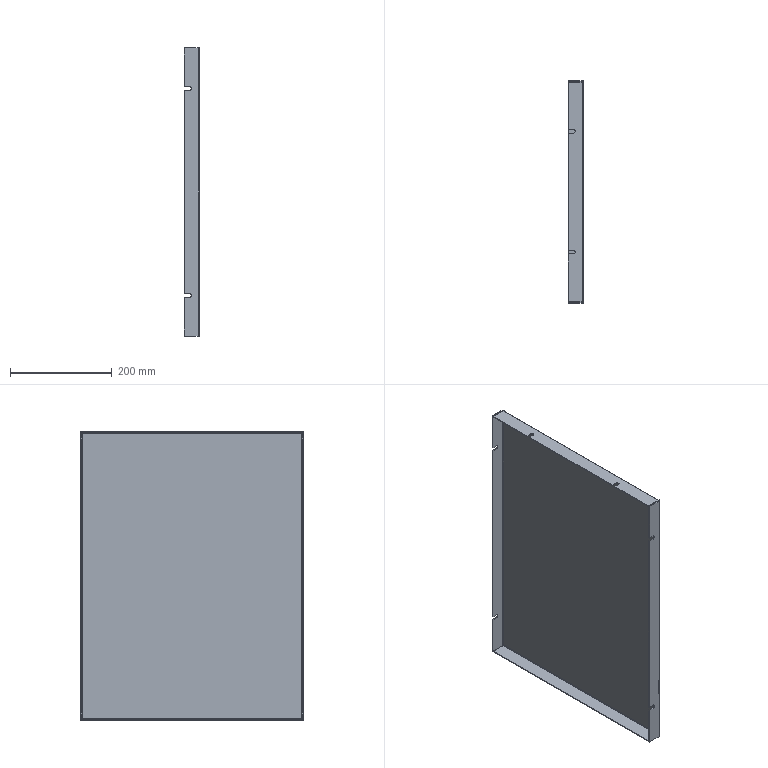Part | STEP file | MEN7-2 | 1 solid | 58 faces | box 30 x 438 x 568 mm | volume 454976 mm3 | plane 44 | cylinder 14 | commonest cylinder face diameters 7 x6 3 x4 6 x4